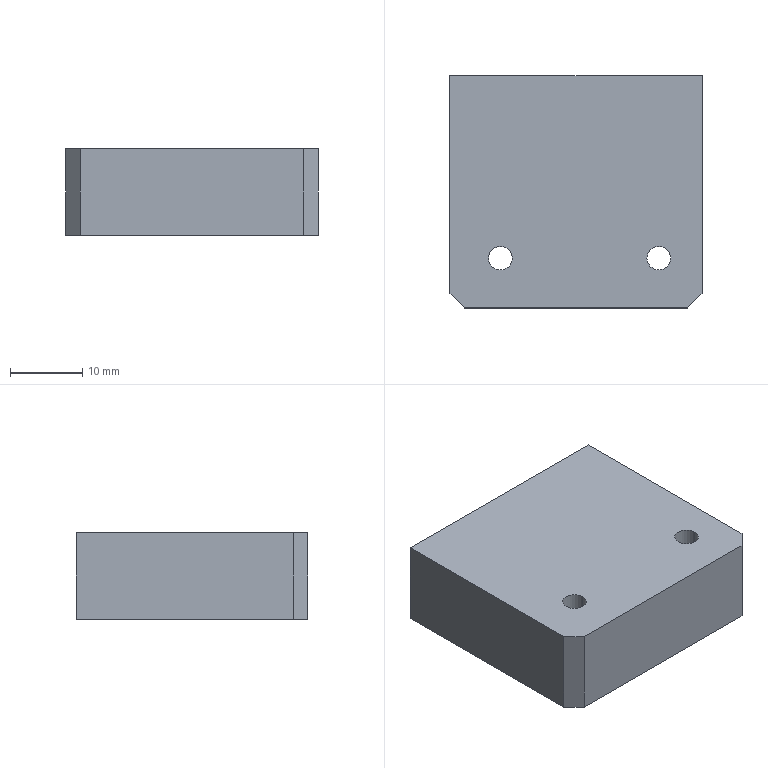Part | SolidWorks | features 3DProfileFeature 2, HoleWzd 2, Chamfer 1, Extrusion 1 | 1 solid | 20 faces | box 35 x 32.2 x 12 mm | volume 12915 mm3 | cylinder 8 | plane 8 | cone 4 | commonest cylinder face diameters 3.3 x4 4.2 x4
STEP:
#1=CARTESIAN_POINT('',(13.15,6.9,6.));
#2=VERTEX_POINT('',#1);
#3=CARTESIAN_POINT('',(9.85,6.9,6.));
#4=VERTEX_POINT('',#3);
#5=CARTESIAN_POINT('',(11.5,6.9,6.));
#6=DIRECTION('',(0.,0.,-1.));
#7=DIRECTION('',(-1.,0.,0.));
#8=AXIS2_PLACEMENT_3D('',#5,#6,#7);
#9=CIRCLE('',#8,1.65);
#10=EDGE_CURVE('',#2,#4,#9,.T.);
#11=ORIENTED_EDGE('',*,*,#10,.F.);
#12=CARTESIAN_POINT('',(13.15,6.9,-6.));
#13=VERTEX_POINT('',#12);
#14=CARTESIAN_POINT('',(13.15,6.9,-6.));
#15=DIRECTION('',(0.,0.,-1.));
#16=VECTOR('',#15,1000.);
#17=LINE('',#14,#16);
#18=EDGE_CURVE('',#2,#13,#17,.T.);
#19=ORIENTED_EDGE('',*,*,#18,.T.);
#20=CARTESIAN_POINT('',(9.85,6.9,-6.));
#21=VERTEX_POINT('',#20);
#22=CARTESIAN_POINT('',(11.5,6.9,-6.));
#23=DIRECTION('',(0.,0.,-1.));
#24=DIRECTION('',(-1.,0.,0.));
#25=AXIS2_PLACEMENT_3D('',#22,#23,#24);
#26=CIRCLE('',#25,1.65);
#27=EDGE_CURVE('',#13,#21,#26,.T.);
#28=ORIENTED_EDGE('',*,*,#27,.T.);
#29=CARTESIAN_POINT('',(9.85,6.9,-6.));
#30=DIRECTION('',(0.,0.,-1.));
#31=VECTOR('',#30,1000.);
#32=LINE('',#29,#31);
#33=EDGE_CURVE('',#4,#21,#32,.T.);
#34=ORIENTED_EDGE('',*,*,#33,.F.);
#35=EDGE_LOOP('',(#11,#19,#28,#34));
#36=FACE_OUTER_BOUND('',#35,.T.);
#37=CARTESIAN_POINT('',(11.5,6.9,-6.));
#38=DIRECTION('',(0.,0.,-1.));
#39=DIRECTION('',(-1.,0.,0.));
#40=AXIS2_PLACEMENT_3D('',#37,#38,#39);
#41=CYLINDRICAL_SURFACE('',#40,1.65);
#42=ADVANCED_FACE('',(#36),#41,.F.);
#43=CARTESIAN_POINT('',(-8.85,6.9,6.));
#44=VERTEX_POINT('',#43);
#45=CARTESIAN_POINT('',(-12.15,6.9,6.));
#46=VERTEX_POINT('',#45);
#47=CARTESIAN_POINT('',(-10.5,6.9,6.));
#48=DIRECTION('',(0.,0.,-1.));
#49=DIRECTION('',(-1.,0.,0.));
#50=AXIS2_PLACEMENT_3D('',#47,#48,#49);
#51=CIRCLE('',#50,1.65);
#52=EDGE_CURVE('',#44,#46,#51,.T.);
#53=ORIENTED_EDGE('',*,*,#52,.F.);
#54=CARTESIAN_POINT('',(-8.85,6.9,-6.));
#55=VERTEX_POINT('',#54);
#56=CARTESIAN_POINT('',(-8.85,6.9,-6.));
#57=DIRECTION('',(0.,0.,-1.));
#58=VECTOR('',#57,1000.);
#59=LINE('',#56,#58);
#60=EDGE_CURVE('',#44,#55,#59,.T.);
#61=ORIENTED_EDGE('',*,*,#60,.T.);
#62=CARTESIAN_POINT('',(-12.15,6.9,-6.));
#63=VERTEX_POINT('',#62);
#64=CARTESIAN_POINT('',(-10.5,6.9,-6.));
#65=DIRECTION('',(0.,0.,-1.));
#66=DIRECTION('',(-1.,0.,0.));
#67=AXIS2_PLACEMENT_3D('',#64,#65,#66);
#68=CIRCLE('',#67,1.65);
#69=EDGE_CURVE('',#55,#63,#68,.T.);
#70=ORIENTED_EDGE('',*,*,#69,.T.);
#71=CARTESIAN_POINT('',(-12.15,6.9,-6.));
#72=DIRECTION('',(0.,0.,-1.));
#73=VECTOR('',#72,1000.);
#74=LINE('',#71,#73);
#75=EDGE_CURVE('',#46,#63,#74,.T.);
#76=ORIENTED_EDGE('',*,*,#75,.F.);
#77=EDGE_LOOP('',(#53,#61,#70,#76));
#78=FACE_OUTER_BOUND('',#77,.T.);
#79=CARTESIAN_POINT('',(-10.5,6.9,-6.));
#80=DIRECTION('',(0.,0.,-1.));
#81=DIRECTION('',(-1.,0.,0.));
#82=AXIS2_PLACEMENT_3D('',#79,#80,#81);
#83=CYLINDRICAL_SURFACE('',#82,1.65);
#84=ADVANCED_FACE('',(#78),#83,.F.);
#85=CARTESIAN_POINT('',(11.5,19.8,-2.1));
#86=VERTEX_POINT('',#85);
#87=CARTESIAN_POINT('',(11.5,19.8,2.1));
#88=VERTEX_POINT('',#87);
#89=CARTESIAN_POINT('',(11.5,19.8,0.));
#90=DIRECTION('',(0.,1.,0.));
#91=DIRECTION('',(0.,0.,1.));
#92=AXIS2_PLACEMENT_3D('',#89,#90,#91);
#93=CIRCLE('',#92,2.1);
#94=EDGE_CURVE('',#86,#88,#93,.T.);
#95=ORIENTED_EDGE('',*,*,#94,.F.);
#96=CARTESIAN_POINT('',(11.5,32.2,-2.1));
#97=VERTEX_POINT('',#96);
#98=CARTESIAN_POINT('',(11.5,32.2,-2.1));
#99=DIRECTION('',(0.,1.,0.));
#100=VECTOR('',#99,1000.);
#101=LINE('',#98,#100);
#102=EDGE_CURVE('',#86,#97,#101,.T.);
#103=ORIENTED_EDGE('',*,*,#102,.T.);
#104=CARTESIAN_POINT('',(11.5,32.2,2.1));
#105=VERTEX_POINT('',#104);
#106=CARTESIAN_POINT('',(11.5,32.2,0.));
#107=DIRECTION('',(0.,1.,0.));
#108=DIRECTION('',(0.,0.,1.));
#109=AXIS2_PLACEMENT_3D('',#106,#107,#108);
#110=CIRCLE('',#109,2.1);
#111=EDGE_CURVE('',#97,#105,#110,.T.);
#112=ORIENTED_EDGE('',*,*,#111,.T.);
#113=CARTESIAN_POINT('',(11.5,32.2,2.1));
#114=DIRECTION('',(0.,1.,0.));
#115=VECTOR('',#114,1000.);
#116=LINE('',#113,#115);
#117=EDGE_CURVE('',#88,#105,#116,.T.);
#118=ORIENTED_EDGE('',*,*,#117,.F.);
#119=EDGE_LOOP('',(#95,#103,#112,#118));
#120=FACE_OUTER_BOUND('',#119,.T.);
#121=CARTESIAN_POINT('',(11.5,32.2,0.));
#122=DIRECTION('',(0.,1.,0.));
#123=DIRECTION('',(0.,0.,1.));
#124=AXIS2_PLACEMENT_3D('',#121,#122,#123);
#125=CYLINDRICAL_SURFACE('',#124,2.1);
#126=ADVANCED_FACE('',(#120),#125,.F.);
#127=CARTESIAN_POINT('',(11.5,18.538,0.));
#128=VERTEX_POINT('',#127);
#129=CARTESIAN_POINT('',(11.5,19.8,2.1));
#130=DIRECTION('',(0.,0.515,0.8572));
#131=VECTOR('',#130,1000.);
#132=LINE('',#129,#131);
#133=EDGE_CURVE('',#128,#88,#132,.T.);
#134=ORIENTED_EDGE('',*,*,#133,.F.);
#135=CARTESIAN_POINT('',(11.5,19.8,-2.1));
#136=DIRECTION('',(0.,0.515,-0.8572));
#137=VECTOR('',#136,1000.);
#138=LINE('',#135,#137);
#139=EDGE_CURVE('',#128,#86,#138,.T.);
#140=ORIENTED_EDGE('',*,*,#139,.T.);
#141=ORIENTED_EDGE('',*,*,#94,.T.);
#142=EDGE_LOOP('',(#134,#140,#141));
#143=FACE_OUTER_BOUND('',#142,.T.);
#144=CARTESIAN_POINT('',(11.5,19.8,0.));
#145=DIRECTION('',(0.,1.,0.));
#146=DIRECTION('',(0.,0.,1.));
#147=AXIS2_PLACEMENT_3D('',#144,#145,#146);
#148=CONICAL_SURFACE('',#147,2.1,1.03);
#149=ADVANCED_FACE('',(#143),#148,.F.);
#150=CARTESIAN_POINT('',(-6.5,19.8,-2.1));
#151=VERTEX_POINT('',#150);
#152=CARTESIAN_POINT('',(-6.5,19.8,2.1));
#153=VERTEX_POINT('',#152);
#154=CARTESIAN_POINT('',(-6.5,19.8,0.));
#155=DIRECTION('',(0.,1.,0.));
#156=DIRECTION('',(0.,0.,1.));
#157=AXIS2_PLACEMENT_3D('',#154,#155,#156);
#158=CIRCLE('',#157,2.1);
#159=EDGE_CURVE('',#151,#153,#158,.T.);
#160=ORIENTED_EDGE('',*,*,#159,.F.);
#161=CARTESIAN_POINT('',(-6.5,32.2,-2.1));
#162=VERTEX_POINT('',#161);
#163=CARTESIAN_POINT('',(-6.5,32.2,-2.1));
#164=DIRECTION('',(0.,1.,0.));
#165=VECTOR('',#164,1000.);
#166=LINE('',#163,#165);
#167=EDGE_CURVE('',#151,#162,#166,.T.);
#168=ORIENTED_EDGE('',*,*,#167,.T.);
#169=CARTESIAN_POINT('',(-6.5,32.2,2.1));
#170=VERTEX_POINT('',#169);
#171=CARTESIAN_POINT('',(-6.5,32.2,0.));
#172=DIRECTION('',(0.,1.,0.));
#173=DIRECTION('',(0.,0.,1.));
#174=AXIS2_PLACEMENT_3D('',#171,#172,#173);
#175=CIRCLE('',#174,2.1);
#176=EDGE_CURVE('',#162,#170,#175,.T.);
#177=ORIENTED_EDGE('',*,*,#176,.T.);
#178=CARTESIAN_POINT('',(-6.5,32.2,2.1));
#179=DIRECTION('',(0.,1.,0.));
#180=VECTOR('',#179,1000.);
#181=LINE('',#178,#180);
#182=EDGE_CURVE('',#153,#170,#181,.T.);
#183=ORIENTED_EDGE('',*,*,#182,.F.);
#184=EDGE_LOOP('',(#160,#168,#177,#183));
#185=FACE_OUTER_BOUND('',#184,.T.);
#186=CARTESIAN_POINT('',(-6.5,32.2,0.));
#187=DIRECTION('',(0.,1.,0.));
#188=DIRECTION('',(0.,0.,1.));
#189=AXIS2_PLACEMENT_3D('',#186,#187,#188);
#190=CYLINDRICAL_SURFACE('',#189,2.1);
#191=ADVANCED_FACE('',(#185),#190,.F.);
#192=CARTESIAN_POINT('',(-6.5,18.538,0.));
#193=VERTEX_POINT('',#192);
#194=CARTESIAN_POINT('',(-6.5,19.8,2.1));
#195=DIRECTION('',(0.,0.515,0.8572));
#196=VECTOR('',#195,1000.);
#197=LINE('',#194,#196);
#198=EDGE_CURVE('',#193,#153,#197,.T.);
#199=ORIENTED_EDGE('',*,*,#198,.F.);
#200=CARTESIAN_POINT('',(-6.5,19.8,-2.1));
#201=DIRECTION('',(0.,0.515,-0.8572));
#202=VECTOR('',#201,1000.);
#203=LINE('',#200,#202);
#204=EDGE_CURVE('',#193,#151,#203,.T.);
#205=ORIENTED_EDGE('',*,*,#204,.T.);
#206=ORIENTED_EDGE('',*,*,#159,.T.);
#207=EDGE_LOOP('',(#199,#205,#206));
#208=FACE_OUTER_BOUND('',#207,.T.);
#209=CARTESIAN_POINT('',(-6.5,19.8,0.));
#210=DIRECTION('',(0.,1.,0.));
#211=DIRECTION('',(0.,0.,1.));
#212=AXIS2_PLACEMENT_3D('',#209,#210,#211);
#213=CONICAL_SURFACE('',#212,2.1,1.03);
#214=ADVANCED_FACE('',(#208),#213,.F.);
#215=CARTESIAN_POINT('',(17.5,32.2,6.));
#216=VERTEX_POINT('',#215);
#217=CARTESIAN_POINT('',(17.5,2.,6.));
#218=VERTEX_POINT('',#217);
#219=CARTESIAN_POINT('',(17.5,32.2,6.));
#220=DIRECTION('',(0.,-1.,0.));
#221=VECTOR('',#220,1000.);
#222=LINE('',#219,#221);
#223=EDGE_CURVE('',#216,#218,#222,.T.);
#224=ORIENTED_EDGE('',*,*,#223,.T.);
#225=CARTESIAN_POINT('',(17.5,2.,-6.));
#226=VERTEX_POINT('',#225);
#227=CARTESIAN_POINT('',(17.5,2.,-6.));
#228=DIRECTION('',(0.,0.,-1.));
#229=VECTOR('',#228,1000.);
#230=LINE('',#227,#229);
#231=EDGE_CURVE('',#218,#226,#230,.T.);
#232=ORIENTED_EDGE('',*,*,#231,.T.);
#233=CARTESIAN_POINT('',(17.5,32.2,-6.));
#234=VERTEX_POINT('',#233);
#235=CARTESIAN_POINT('',(17.5,32.2,-6.));
#236=DIRECTION('',(0.,-1.,0.));
#237=VECTOR('',#236,1000.);
#238=LINE('',#235,#237);
#239=EDGE_CURVE('',#234,#226,#238,.T.);
#240=ORIENTED_EDGE('',*,*,#239,.F.);
#241=CARTESIAN_POINT('',(17.5,32.2,-6.));
#242=DIRECTION('',(0.,0.,-1.));
#243=VECTOR('',#242,1000.);
#244=LINE('',#241,#243);
#245=EDGE_CURVE('',#216,#234,#244,.T.);
#246=ORIENTED_EDGE('',*,*,#245,.F.);
#247=EDGE_LOOP('',(#224,#232,#240,#246));
#248=FACE_OUTER_BOUND('',#247,.T.);
#249=CARTESIAN_POINT('',(17.5,32.2,-6.));
#250=DIRECTION('',(-1.,0.,0.));
#251=DIRECTION('',(0.,0.,1.));
#252=AXIS2_PLACEMENT_3D('',#249,#250,#251);
#253=PLANE('',#252);
#254=ADVANCED_FACE('',(#248),#253,.F.);
#255=CARTESIAN_POINT('',(11.5,6.9,-6.));
#256=DIRECTION('',(0.,0.,-1.));
#257=DIRECTION('',(-1.,0.,0.));
#258=AXIS2_PLACEMENT_3D('',#255,#256,#257);
#259=CIRCLE('',#258,1.65);
#260=EDGE_CURVE('',#21,#13,#259,.T.);
#261=ORIENTED_EDGE('',*,*,#260,.F.);
#262=ORIENTED_EDGE('',*,*,#27,.F.);
#263=EDGE_LOOP('',(#261,#262));
#264=FACE_BOUND('',#263,.T.);
#265=CARTESIAN_POINT('',(-10.5,6.9,-6.));
#266=DIRECTION('',(0.,0.,-1.));
#267=DIRECTION('',(-1.,0.,0.));
#268=AXIS2_PLACEMENT_3D('',#265,#266,#267);
#269=CIRCLE('',#268,1.65);
#270=EDGE_CURVE('',#63,#55,#269,.T.);
#271=ORIENTED_EDGE('',*,*,#270,.F.);
#272=ORIENTED_EDGE('',*,*,#69,.F.);
#273=EDGE_LOOP('',(#271,#272));
#274=FACE_BOUND('',#273,.T.);
#275=ORIENTED_EDGE('',*,*,#239,.T.);
#276=CARTESIAN_POINT('',(15.5,0.,-6.));
#277=VERTEX_POINT('',#276);
#278=CARTESIAN_POINT('',(17.5,2.,-6.));
#279=DIRECTION('',(-0.7071,-0.7071,0.));
#280=VECTOR('',#279,1000.);
#281=LINE('',#278,#280);
#282=EDGE_CURVE('',#226,#277,#281,.T.);
#283=ORIENTED_EDGE('',*,*,#282,.T.);
#284=CARTESIAN_POINT('',(-15.5,0.,-6.));
#285=VERTEX_POINT('',#284);
#286=CARTESIAN_POINT('',(-17.5,0.,-6.));
#287=DIRECTION('',(-1.,0.,0.));
#288=VECTOR('',#287,1000.);
#289=LINE('',#286,#288);
#290=EDGE_CURVE('',#277,#285,#289,.T.);
#291=ORIENTED_EDGE('',*,*,#290,.T.);
#292=CARTESIAN_POINT('',(-17.5,2.,-6.));
#293=VERTEX_POINT('',#292);
#294=CARTESIAN_POINT('',(-17.5,2.,-6.));
#295=DIRECTION('',(-0.7071,0.7071,0.));
#296=VECTOR('',#295,1000.);
#297=LINE('',#294,#296);
#298=EDGE_CURVE('',#285,#293,#297,.T.);
#299=ORIENTED_EDGE('',*,*,#298,.T.);
#300=CARTESIAN_POINT('',(-17.5,32.2,-6.));
#301=VERTEX_POINT('',#300);
#302=CARTESIAN_POINT('',(-17.5,32.2,-6.));
#303=DIRECTION('',(0.,-1.,0.));
#304=VECTOR('',#303,1000.);
#305=LINE('',#302,#304);
#306=EDGE_CURVE('',#301,#293,#305,.T.);
#307=ORIENTED_EDGE('',*,*,#306,.F.);
#308=CARTESIAN_POINT('',(-17.5,32.2,-6.));
#309=DIRECTION('',(-1.,0.,0.));
#310=VECTOR('',#309,1000.);
#311=LINE('',#308,#310);
#312=EDGE_CURVE('',#234,#301,#311,.T.);
#313=ORIENTED_EDGE('',*,*,#312,.F.);
#314=EDGE_LOOP('',(#275,#283,#291,#299,#307,#313));
#315=FACE_OUTER_BOUND('',#314,.T.);
#316=CARTESIAN_POINT('',(-17.5,32.2,-6.));
#317=DIRECTION('',(0.,0.,1.));
#318=DIRECTION('',(1.,0.,0.));
#319=AXIS2_PLACEMENT_3D('',#316,#317,#318);
#320=PLANE('',#319);
#321=ADVANCED_FACE('',(#264,#274,#315),#320,.F.);
#322=ORIENTED_EDGE('',*,*,#306,.T.);
#323=CARTESIAN_POINT('',(-17.5,2.,6.));
#324=VERTEX_POINT('',#323);
#325=CARTESIAN_POINT('',(-17.5,2.,-6.));
#326=DIRECTION('',(0.,0.,1.));
#327=VECTOR('',#326,1000.);
#328=LINE('',#325,#327);
#329=EDGE_CURVE('',#293,#324,#328,.T.);
#330=ORIENTED_EDGE('',*,*,#329,.T.);
#331=CARTESIAN_POINT('',(-17.5,32.2,6.));
#332=VERTEX_POINT('',#331);
#333=CARTESIAN_POINT('',(-17.5,32.2,6.));
#334=DIRECTION('',(0.,-1.,0.));
#335=VECTOR('',#334,1000.);
#336=LINE('',#333,#335);
#337=EDGE_CURVE('',#332,#324,#336,.T.);
#338=ORIENTED_EDGE('',*,*,#337,.F.);
#339=CARTESIAN_POINT('',(-17.5,32.2,-6.));
#340=DIRECTION('',(0.,0.,1.));
#341=VECTOR('',#340,1000.);
#342=LINE('',#339,#341);
#343=EDGE_CURVE('',#301,#332,#342,.T.);
#344=ORIENTED_EDGE('',*,*,#343,.F.);
#345=EDGE_LOOP('',(#322,#330,#338,#344));
#346=FACE_OUTER_BOUND('',#345,.T.);
#347=CARTESIAN_POINT('',(-17.5,32.2,-6.));
#348=DIRECTION('',(1.,0.,0.));
#349=DIRECTION('',(0.,0.,-1.));
#350=AXIS2_PLACEMENT_3D('',#347,#348,#349);
#351=PLANE('',#350);
#352=ADVANCED_FACE('',(#346),#351,.F.);
#353=CARTESIAN_POINT('',(11.5,6.9,6.));
#354=DIRECTION('',(0.,0.,-1.));
#355=DIRECTION('',(-1.,0.,0.));
#356=AXIS2_PLACEMENT_3D('',#353,#354,#355);
#357=CIRCLE('',#356,1.65);
#358=EDGE_CURVE('',#4,#2,#357,.T.);
#359=ORIENTED_EDGE('',*,*,#358,.T.);
#360=ORIENTED_EDGE('',*,*,#10,.T.);
#361=EDGE_LOOP('',(#359,#360));
#362=FACE_BOUND('',#361,.T.);
#363=CARTESIAN_POINT('',(-10.5,6.9,6.));
#364=DIRECTION('',(0.,0.,-1.));
#365=DIRECTION('',(-1.,0.,0.));
#366=AXIS2_PLACEMENT_3D('',#363,#364,#365);
#367=CIRCLE('',#366,1.65);
#368=EDGE_CURVE('',#46,#44,#367,.T.);
#369=ORIENTED_EDGE('',*,*,#368,.T.);
#370=ORIENTED_EDGE('',*,*,#52,.T.);
#371=EDGE_LOOP('',(#369,#370));
#372=FACE_BOUND('',#371,.T.);
#373=CARTESIAN_POINT('',(-15.5,0.,6.));
#374=VERTEX_POINT('',#373);
#375=CARTESIAN_POINT('',(15.5,0.,6.));
#376=VERTEX_POINT('',#375);
#377=CARTESIAN_POINT('',(-17.5,0.,6.));
#378=DIRECTION('',(1.,0.,0.));
#379=VECTOR('',#378,1000.);
#380=LINE('',#377,#379);
#381=EDGE_CURVE('',#374,#376,#380,.T.);
#382=ORIENTED_EDGE('',*,*,#381,.T.);
#383=CARTESIAN_POINT('',(17.5,2.,6.));
#384=DIRECTION('',(0.7071,0.7071,0.));
#385=VECTOR('',#384,1000.);
#386=LINE('',#383,#385);
#387=EDGE_CURVE('',#376,#218,#386,.T.);
#388=ORIENTED_EDGE('',*,*,#387,.T.);
#389=ORIENTED_EDGE('',*,*,#223,.F.);
#390=CARTESIAN_POINT('',(-17.5,32.2,6.));
#391=DIRECTION('',(1.,0.,0.));
#392=VECTOR('',#391,1000.);
#393=LINE('',#390,#392);
#394=EDGE_CURVE('',#332,#216,#393,.T.);
#395=ORIENTED_EDGE('',*,*,#394,.F.);
#396=ORIENTED_EDGE('',*,*,#337,.T.);
#397=CARTESIAN_POINT('',(-17.5,2.,6.));
#398=DIRECTION('',(0.7071,-0.7071,0.));
#399=VECTOR('',#398,1000.);
#400=LINE('',#397,#399);
#401=EDGE_CURVE('',#324,#374,#400,.T.);
#402=ORIENTED_EDGE('',*,*,#401,.T.);
#403=EDGE_LOOP('',(#382,#388,#389,#395,#396,#402));
#404=FACE_OUTER_BOUND('',#403,.T.);
#405=CARTESIAN_POINT('',(-17.5,32.2,6.));
#406=DIRECTION('',(0.,0.,-1.));
#407=DIRECTION('',(-1.,0.,0.));
#408=AXIS2_PLACEMENT_3D('',#405,#406,#407);
#409=PLANE('',#408);
#410=ADVANCED_FACE('',(#362,#372,#404),#409,.F.);
#411=CARTESIAN_POINT('',(11.5,32.2,0.));
#412=DIRECTION('',(0.,1.,0.));
#413=DIRECTION('',(0.,0.,1.));
#414=AXIS2_PLACEMENT_3D('',#411,#412,#413);
#415=CIRCLE('',#414,2.1);
#416=EDGE_CURVE('',#105,#97,#415,.T.);
#417=ORIENTED_EDGE('',*,*,#416,.F.);
#418=ORIENTED_EDGE('',*,*,#111,.F.);
#419=EDGE_LOOP('',(#417,#418));
#420=FACE_BOUND('',#419,.T.);
#421=CARTESIAN_POINT('',(-6.5,32.2,0.));
#422=DIRECTION('',(0.,1.,0.));
#423=DIRECTION('',(0.,0.,1.));
#424=AXIS2_PLACEMENT_3D('',#421,#422,#423);
#425=CIRCLE('',#424,2.1);
#426=EDGE_CURVE('',#170,#162,#425,.T.);
#427=ORIENTED_EDGE('',*,*,#426,.F.);
#428=ORIENTED_EDGE('',*,*,#176,.F.);
#429=EDGE_LOOP('',(#427,#428));
#430=FACE_BOUND('',#429,.T.);
#431=ORIENTED_EDGE('',*,*,#245,.T.);
#432=ORIENTED_EDGE('',*,*,#312,.T.);
#433=ORIENTED_EDGE('',*,*,#343,.T.);
#434=ORIENTED_EDGE('',*,*,#394,.T.);
#435=EDGE_LOOP('',(#431,#432,#433,#434));
#436=FACE_OUTER_BOUND('',#435,.T.);
#437=CARTESIAN_POINT('',(0.,32.2,0.));
#438=DIRECTION('',(0.,1.,0.));
#439=DIRECTION('',(0.,0.,1.));
#440=AXIS2_PLACEMENT_3D('',#437,#438,#439);
#441=PLANE('',#440);
#442=ADVANCED_FACE('',(#420,#430,#436),#441,.T.);
#443=ORIENTED_EDGE('',*,*,#290,.F.);
#444=CARTESIAN_POINT('',(15.5,0.,0.));
#445=DIRECTION('',(0.,0.,1.));
#446=VECTOR('',#445,1000.);
#447=LINE('',#444,#446);
#448=EDGE_CURVE('',#277,#376,#447,.T.);
#449=ORIENTED_EDGE('',*,*,#448,.T.);
#450=ORIENTED_EDGE('',*,*,#381,.F.);
#451=CARTESIAN_POINT('',(-15.5,0.,0.));
#452=DIRECTION('',(0.,0.,-1.));
#453=VECTOR('',#452,1000.);
#454=LINE('',#451,#453);
#455=EDGE_CURVE('',#374,#285,#454,.T.);
#456=ORIENTED_EDGE('',*,*,#455,.T.);
#457=EDGE_LOOP('',(#443,#449,#450,#456));
#458=FACE_OUTER_BOUND('',#457,.T.);
#459=CARTESIAN_POINT('',(0.,0.,0.));
#460=DIRECTION('',(0.,1.,0.));
#461=DIRECTION('',(0.,0.,1.));
#462=AXIS2_PLACEMENT_3D('',#459,#460,#461);
#463=PLANE('',#462);
#464=ADVANCED_FACE('',(#458),#463,.F.);
#465=ORIENTED_EDGE('',*,*,#204,.F.);
#466=ORIENTED_EDGE('',*,*,#198,.T.);
#467=CARTESIAN_POINT('',(-6.5,19.8,0.));
#468=DIRECTION('',(0.,1.,0.));
#469=DIRECTION('',(0.,0.,1.));
#470=AXIS2_PLACEMENT_3D('',#467,#468,#469);
#471=CIRCLE('',#470,2.1);
#472=EDGE_CURVE('',#153,#151,#471,.T.);
#473=ORIENTED_EDGE('',*,*,#472,.T.);
#474=EDGE_LOOP('',(#465,#466,#473));
#475=FACE_OUTER_BOUND('',#474,.T.);
#476=CARTESIAN_POINT('',(-6.5,19.8,0.));
#477=DIRECTION('',(0.,1.,0.));
#478=DIRECTION('',(0.,0.,1.));
#479=AXIS2_PLACEMENT_3D('',#476,#477,#478);
#480=CONICAL_SURFACE('',#479,2.1,1.03);
#481=ADVANCED_FACE('',(#475),#480,.F.);
#482=ORIENTED_EDGE('',*,*,#167,.F.);
#483=ORIENTED_EDGE('',*,*,#472,.F.);
#484=ORIENTED_EDGE('',*,*,#182,.T.);
#485=ORIENTED_EDGE('',*,*,#426,.T.);
#486=EDGE_LOOP('',(#482,#483,#484,#485));
#487=FACE_OUTER_BOUND('',#486,.T.);
#488=CARTESIAN_POINT('',(-6.5,32.2,0.));
#489=DIRECTION('',(0.,1.,0.));
#490=DIRECTION('',(0.,0.,1.));
#491=AXIS2_PLACEMENT_3D('',#488,#489,#490);
#492=CYLINDRICAL_SURFACE('',#491,2.1);
#493=ADVANCED_FACE('',(#487),#492,.F.);
#494=ORIENTED_EDGE('',*,*,#139,.F.);
#495=ORIENTED_EDGE('',*,*,#133,.T.);
#496=CARTESIAN_POINT('',(11.5,19.8,0.));
#497=DIRECTION('',(0.,1.,0.));
#498=DIRECTION('',(0.,0.,1.));
#499=AXIS2_PLACEMENT_3D('',#496,#497,#498);
#500=CIRCLE('',#499,2.1);
#501=EDGE_CURVE('',#88,#86,#500,.T.);
#502=ORIENTED_EDGE('',*,*,#501,.T.);
#503=EDGE_LOOP('',(#494,#495,#502));
#504=FACE_OUTER_BOUND('',#503,.T.);
#505=CARTESIAN_POINT('',(11.5,19.8,0.));
#506=DIRECTION('',(0.,1.,0.));
#507=DIRECTION('',(0.,0.,1.));
#508=AXIS2_PLACEMENT_3D('',#505,#506,#507);
#509=CONICAL_SURFACE('',#508,2.1,1.03);
#510=ADVANCED_FACE('',(#504),#509,.F.);
#511=ORIENTED_EDGE('',*,*,#102,.F.);
#512=ORIENTED_EDGE('',*,*,#501,.F.);
#513=ORIENTED_EDGE('',*,*,#117,.T.);
#514=ORIENTED_EDGE('',*,*,#416,.T.);
#515=EDGE_LOOP('',(#511,#512,#513,#514));
#516=FACE_OUTER_BOUND('',#515,.T.);
#517=CARTESIAN_POINT('',(11.5,32.2,0.));
#518=DIRECTION('',(0.,1.,0.));
#519=DIRECTION('',(0.,0.,1.));
#520=AXIS2_PLACEMENT_3D('',#517,#518,#519);
#521=CYLINDRICAL_SURFACE('',#520,2.1);
#522=ADVANCED_FACE('',(#516),#521,.F.);
#523=ORIENTED_EDGE('',*,*,#387,.F.);
#524=ORIENTED_EDGE('',*,*,#448,.F.);
#525=ORIENTED_EDGE('',*,*,#282,.F.);
#526=ORIENTED_EDGE('',*,*,#231,.F.);
#527=EDGE_LOOP('',(#523,#524,#525,#526));
#528=FACE_OUTER_BOUND('',#527,.T.);
#529=CARTESIAN_POINT('',(17.5,2.,-6.));
#530=DIRECTION('',(-0.7071,0.7071,0.));
#531=DIRECTION('',(0.,0.,-1.));
#532=AXIS2_PLACEMENT_3D('',#529,#530,#531);
#533=PLANE('',#532);
#534=ADVANCED_FACE('',(#528),#533,.F.);
#535=ORIENTED_EDGE('',*,*,#298,.F.);
#536=ORIENTED_EDGE('',*,*,#455,.F.);
#537=ORIENTED_EDGE('',*,*,#401,.F.);
#538=ORIENTED_EDGE('',*,*,#329,.F.);
#539=EDGE_LOOP('',(#535,#536,#537,#538));
#540=FACE_OUTER_BOUND('',#539,.T.);
#541=CARTESIAN_POINT('',(-17.5,2.,-6.));
#542=DIRECTION('',(0.7071,0.7071,0.));
#543=DIRECTION('',(0.,0.,1.));
#544=AXIS2_PLACEMENT_3D('',#541,#542,#543);
#545=PLANE('',#544);
#546=ADVANCED_FACE('',(#540),#545,.F.);
#547=ORIENTED_EDGE('',*,*,#60,.F.);
#548=ORIENTED_EDGE('',*,*,#368,.F.);
#549=ORIENTED_EDGE('',*,*,#75,.T.);
#550=ORIENTED_EDGE('',*,*,#270,.T.);
#551=EDGE_LOOP('',(#547,#548,#549,#550));
#552=FACE_OUTER_BOUND('',#551,.T.);
#553=CARTESIAN_POINT('',(-10.5,6.9,-6.));
#554=DIRECTION('',(0.,0.,-1.));
#555=DIRECTION('',(-1.,0.,0.));
#556=AXIS2_PLACEMENT_3D('',#553,#554,#555);
#557=CYLINDRICAL_SURFACE('',#556,1.65);
#558=ADVANCED_FACE('',(#552),#557,.F.);
#559=ORIENTED_EDGE('',*,*,#18,.F.);
#560=ORIENTED_EDGE('',*,*,#358,.F.);
#561=ORIENTED_EDGE('',*,*,#33,.T.);
#562=ORIENTED_EDGE('',*,*,#260,.T.);
#563=EDGE_LOOP('',(#559,#560,#561,#562));
#564=FACE_OUTER_BOUND('',#563,.T.);
#565=CARTESIAN_POINT('',(11.5,6.9,-6.));
#566=DIRECTION('',(0.,0.,-1.));
#567=DIRECTION('',(-1.,0.,0.));
#568=AXIS2_PLACEMENT_3D('',#565,#566,#567);
#569=CYLINDRICAL_SURFACE('',#568,1.65);
#570=ADVANCED_FACE('',(#564),#569,.F.);
#571=CLOSED_SHELL('',(#42,#84,#126,#149,#191,#214,#254,#321,#352,#410,#442,#464,#481,#493,#510,#522,#534,#546,#558,#570));
#572=MANIFOLD_SOLID_BREP('',#571);
#573=CARTESIAN_POINT('',(0.,0.,0.));
#574=DIRECTION('',(0.,0.,1.));
#575=DIRECTION('',(1.,0.,0.));
#576=AXIS2_PLACEMENT_3D('',#573,#574,#575);
#577=(LENGTH_UNIT()NAMED_UNIT(*)SI_UNIT(.MILLI.,.METRE.));
#578=UNCERTAINTY_MEASURE_WITH_UNIT(LENGTH_MEASURE(0.00001),#577,'','');
#579=(NAMED_UNIT(*)PLANE_ANGLE_UNIT()SI_UNIT($,.RADIAN.));
#580=(NAMED_UNIT(*)SI_UNIT($,.STERADIAN.)SOLID_ANGLE_UNIT());
#581=(GEOMETRIC_REPRESENTATION_CONTEXT(3)GLOBAL_UNCERTAINTY_ASSIGNED_CONTEXT((#578))GLOBAL_UNIT_ASSIGNED_CONTEXT((#577,#579,#580))REPRESENTATION_CONTEXT('',''));
#582=ADVANCED_BREP_SHAPE_REPRESENTATION('',(#572,#576),#581);